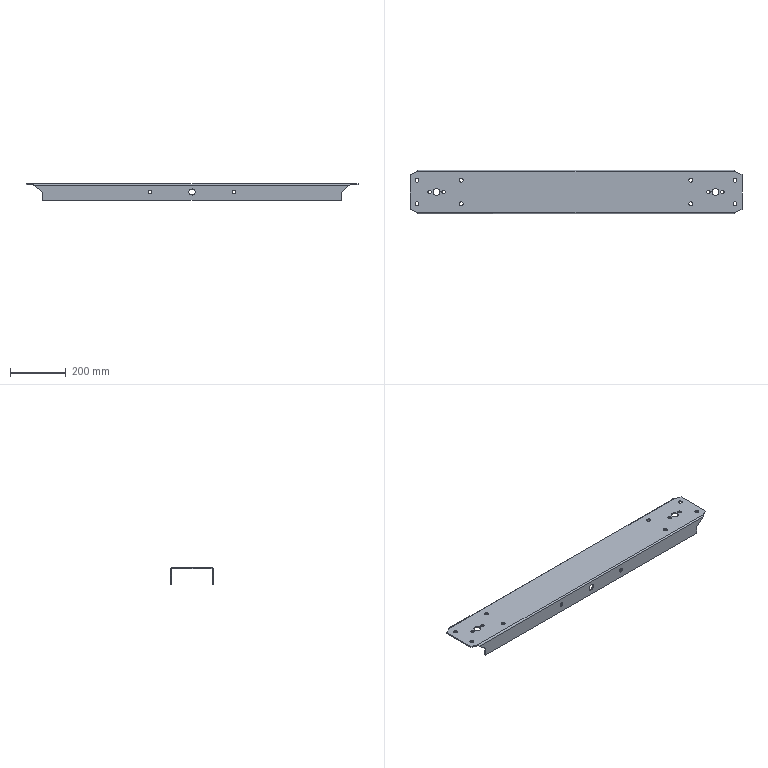Part | 1 solid | 86 faces | box 1186 x 154 x 60 mm | volume 1179056 mm3 | cylinder 52 | plane 30 | spline 4 | commonest cylinder face diameters 14 x32 12 x8 22 x4 25 x4 2 x2 10 x2